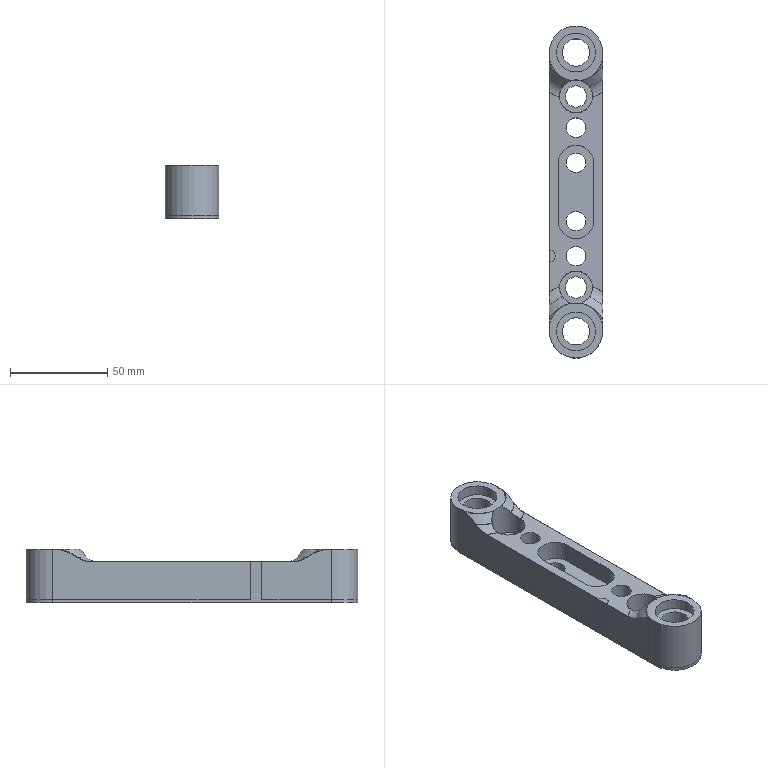NC program | NX | posted with a generic post | part box 27.4 x 170.48 x 27.5 mm
Lines 378 to 1221 of 16455:
(CURVE_DRIVE , TOOL : R3)
N688 T10 M6
N690 G54
N692 G17 G0 G90 X49.499 Y5.551 B0. C0. S4000 M3
N694 G43 Z30. H10
N696 Z-3.399
N698 G94 G1 Z-3.614 F1500.
N700 X49.462 Y5.673 Z-4.386
N702 X49.369 Y5.983 Z-5.1
N704 X49.226 Y6.459 Z-5.705
N706 X49.043 Y7.069 Z-6.161
N708 X48.832 Y7.771 Z-6.437
N710 X48.608 Y8.517 Z-6.513
N712 X48.584 Y8.595 Z-6.51
N714 X48.613 Y8.669 Z-6.507
N716 X48.657 Y8.524 Z-6.511
N718 X48.707 Y8.53 Z-6.51
N720 X48.643 Y8.744 Z-6.505
N722 X48.672 Y8.818 Z-6.502
N724 X48.756 Y8.537 Z-6.508
N726 X48.806 Y8.543 Z-6.507
N728 X48.701 Y8.893 Z-6.499
N730 X48.73 Y8.967
N732 X48.856 Y8.549 Z-6.506
N734 X48.905 Y8.555 Z-6.504
N736 X48.804 Y8.892 Z-6.496
N738 X48.759 Y9.041 Z-6.499
N740 X48.788 Y9.115 Z-6.498
N742 X48.854 Y8.892 Z-6.494
N744 X48.955 Y8.559 Z-6.498
N746 X49.004 Y8.561 Z-6.49
N748 X48.816 Y9.187 Z-6.498
N750 X48.845 Y9.256
N752 X49.053 Y8.564 Z-6.483
N754 X49.103 Y8.566 Z-6.476
N756 X49.042 Y8.769 Z-6.478
N758 X48.922 Y9.166 Z-6.495
N760 X48.875 Y9.324 Z-6.498
N762 X48.904 Y9.393
N764 X49.055 Y8.892 Z-6.482
N766 X49.114 Y8.696 Z-6.47
N768 X49.152 Y8.568 Z-6.468
N770 X49.202 Y8.571 Z-6.461
N772 X48.978 Y9.313 Z-6.494
N774 X48.934 Y9.461 Z-6.497
N776 X48.964 Y9.529
N778 X49.066 Y9.188 Z-6.489
N780 X49.251 Y8.573 Z-6.454
N782 X49.301 Y8.575 Z-6.451
N784 X49.098 Y9.252 Z-6.488
N786 X48.993 Y9.598 Z-6.497
N788 X49.023 Y9.667
N790 X49.129 Y9.315 Z-6.488
N792 X49.333 Y8.637 Z-6.451
N794 X49.351 Y8.578 Z-6.445
N796 X49.4 Y8.58 Z-6.436
N798 X49.306 Y8.892 Z-6.464
N800 X49.16 Y9.378 Z-6.487
N802 X49.053 Y9.735 Z-6.496
N804 X49.082 Y9.803
N806 X49.191 Y9.441 Z-6.486
N808 X49.356 Y8.892 Z-6.457
N810 X49.449 Y8.583 Z-6.427
N812 X49.498 Y8.586 Z-6.418
N814 X49.378 Y8.984 Z-6.46
N816 X49.155 Y9.727 Z-6.491
N818 X49.112 Y9.871 Z-6.496
N820 X49.141 Y9.939
N822 X49.253 Y9.566 Z-6.485
N824 X49.409 Y9.047 Z-6.459
N826 X49.547 Y8.588 Z-6.409
N828 X49.595 Y8.591 Z-6.4
N830 X49.504 Y8.892 Z-6.43
N832 X49.439 Y9.108 Z-6.459
N834 X49.253 Y9.727 Z-6.487
N836 X49.17 Y10.005 Z-6.496
N838 X49.198 Y10.069
N840 X49.469 Y9.168 Z-6.458
N842 X49.552 Y8.892 Z-6.421
N844 X49.642 Y8.594 Z-6.39
N846 X49.689 Y8.596 Z-6.38
N848 X49.499 Y9.228 Z-6.457
N850 X49.227 Y10.13 Z-6.496
N852 X49.256 Y10.192
N854 X49.396 Y9.727 Z-6.478
N856 X49.528 Y9.287 Z-6.456
N858 X49.647 Y8.892 Z-6.404
N860 X49.735 Y8.599 Z-6.37
N862 X49.782 Y8.598 Z-6.36
N864 X49.755 Y8.688 Z-6.375
N866 X49.693 Y8.892 Z-6.395
N868 X49.557 Y9.346 Z-6.455
N870 X49.401 Y9.865 Z-6.483
N872 X49.285 Y10.252 Z-6.496
N874 X49.313 Y10.312
N876 X49.429 Y9.923 Z-6.483
N878 X49.586 Y9.404 Z-6.454
N880 X49.739 Y8.892 Z-6.387
N882 X49.795 Y8.708 Z-6.369
N884 X49.83 Y8.59 Z-6.349
N886 X49.878 Y8.583 Z-6.338
N888 X49.834 Y8.729 Z-6.362
N890 X49.785 Y8.892 Z-6.378
N892 X49.614 Y9.462 Z-6.454
N894 X49.458 Y9.981 Z-6.483
N896 X49.341 Y10.372 Z-6.496
N898 X49.368 Y10.431
N900 X49.486 Y10.038 Z-6.483
N902 X49.642 Y9.519 Z-6.453
N904 X49.831 Y8.892 Z-6.37
N906 X49.874 Y8.749 Z-6.356
N908 X49.926 Y8.575 Z-6.327
N910 X49.973 Y8.568 Z-6.316
N912 X49.913 Y8.768 Z-6.349
N914 X49.67 Y9.576 Z-6.452
N916 X49.514 Y10.095 Z-6.483
N918 X49.396 Y10.49 Z-6.496
N920 X49.423 Y10.548
N922 X49.542 Y10.151 Z-6.483
N924 X49.698 Y9.632 Z-6.451
N926 X49.952 Y8.788 Z-6.343
N928 X50.02 Y8.561 Z-6.305
N930 X50.067 Y8.554 Z-6.294
N932 X49.99 Y8.808 Z-6.337
N934 X49.714 Y9.727 Z-6.452
N936 X49.57 Y10.207 Z-6.483
N938 X49.45 Y10.605 Z-6.496
N940 X49.477 Y10.662
N942 X49.597 Y10.263 Z-6.482
N944 X49.758 Y9.727 Z-6.448
N946 X50.029 Y8.827 Z-6.33
N948 X50.113 Y8.546 Z-6.283
N950 X50.158 Y8.539 Z-6.273
N952 X50.052 Y8.892 Z-6.329
N954 X49.78 Y9.798 Z-6.45
N956 X49.624 Y10.317 Z-6.482
N958 X49.503 Y10.719 Z-6.496
N960 X49.53 Y10.775
N962 X49.651 Y10.371 Z-6.482
N964 X49.807 Y9.852 Z-6.449
N966 X50.104 Y8.865 Z-6.318
N968 X50.204 Y8.532 Z-6.258
N970 X50.248 Y8.526 Z-6.24
N972 X50.141 Y8.884 Z-6.312
N974 X49.887 Y9.727 Z-6.429
N976 X49.834 Y9.906 Z-6.449
N978 X49.677 Y10.425 Z-6.482
N980 X49.556 Y10.83 Z-6.496
N982 X49.582 Y10.885
N984 X49.704 Y10.478 Z-6.482
N986 X49.86 Y9.959 Z-6.449
N988 X49.93 Y9.727 Z-6.423
N990 X50.181 Y8.892 Z-6.302
N992 X50.272 Y8.59 Z-6.243
N994 X50.293 Y8.519 Z-6.224
N996 X50.337 Y8.513 Z-6.208
N998 X50.304 Y8.623 Z-6.236
N1000 X50.158 Y9.109 Z-6.33
N1002 X49.972 Y9.727 Z-6.417
N1004 X49.886 Y10.013 Z-6.449
N1006 X49.73 Y10.532 Z-6.482
N1008 X49.608 Y10.939 Z-6.496
N1010 X49.635 Y10.993
N1012 X49.757 Y10.586 Z-6.482
N1014 X49.913 Y10.067 Z-6.449
N1016 X50.015 Y9.727 Z-6.411
N1018 X50.158 Y9.252 Z-6.344
N1020 X50.337 Y8.656 Z-6.23
N1022 X50.361 Y8.577 Z-6.206
N1024 X50.382 Y8.506 Z-6.192
N1026 X50.428 Y8.5 Z-6.176
N1028 X50.399 Y8.597 Z-6.194
N1030 X50.371 Y8.69 Z-6.223
N1032 X50.158 Y9.397 Z-6.358
N1034 X50.059 Y9.727 Z-6.405
N1036 X49.94 Y10.122 Z-6.449
N1038 X49.784 Y10.641 Z-6.482
N1040 X49.662 Y11.047 Z-6.496
N1042 X49.689 Y11.102
N1044 X49.852 Y10.563 Z-6.473
N1046 X49.968 Y10.177 Z-6.448
N1048 X50.103 Y9.727 Z-6.398
N1050 X50.158 Y9.543 Z-6.372
N1052 X50.404 Y8.724 Z-6.216
N1054 X50.437 Y8.616 Z-6.183
N1056 X50.474 Y8.493 Z-6.16
N1058 X50.52 Y8.486 Z-6.144
N1060 X50.475 Y8.635 Z-6.172
N1062 X50.438 Y8.758 Z-6.209
N1064 X50.147 Y9.727 Z-6.392
N1066 X49.995 Y10.232 Z-6.448
N1068 X49.839 Y10.752 Z-6.482
N1070 X49.717 Y11.158 Z-6.497
N1072 X49.744 Y11.214
N1074 X49.866 Y10.807 Z-6.482
N1076 X50.023 Y10.288 Z-6.448
N1078 X50.191 Y9.727 Z-6.382
N1080 X50.472 Y8.792 Z-6.202
N1082 X50.514 Y8.655 Z-6.16
N1084 X50.566 Y8.479 Z-6.128
N1086 X50.612 Y8.473 Z-6.111
N1088 X50.552 Y8.674 Z-6.148
N1090 X50.506 Y8.827 Z-6.195
N1092 X50.218 Y9.788 Z-6.383
N1094 X50.05 Y10.344 Z-6.448
N1096 X49.894 Y10.864 Z-6.482
N1098 X49.772 Y11.269 Z-6.497
N1100 X49.802 Y11.324 Z-6.496
N1102 X49.923 Y10.922 Z-6.482
N1104 X50.079 Y10.403 Z-6.448
N1106 X50.253 Y9.824 Z-6.379
N1108 X50.542 Y8.863 Z-6.188
N1110 X50.593 Y8.695 Z-6.136
N1112 X50.664 Y8.457 Z-6.092
N1114 X50.716 Y8.442 Z-6.073
N1116 X50.634 Y8.716 Z-6.124
N1118 X50.577 Y8.905 Z-6.182
N1120 X50.29 Y9.861 Z-6.375
N1122 X50.109 Y10.463 Z-6.447
N1124 X49.953 Y10.982 Z-6.482
N1126 X49.833 Y11.381 Z-6.496
N1128 X49.864 Y11.44
N1130 X49.983 Y11.044 Z-6.482
N1132 X50.158 Y10.463 Z-6.44
N1134 X50.328 Y9.899 Z-6.371
N1136 X50.379 Y9.727 Z-6.331
N1138 X50.608 Y8.967 Z-6.181
N1140 X50.677 Y8.737 Z-6.111
N1142 X50.77 Y8.426 Z-6.051
N1144 X50.824 Y8.411 Z-6.021
N1146 X50.794 Y8.51 Z-6.052
N1148 X50.72 Y8.759 Z-6.098
N1150 X50.638 Y9.029 Z-6.18
N1152 X50.428 Y9.727 Z-6.318
N1154 X50.365 Y9.937 Z-6.366
N1156 X50.17 Y10.587 Z-6.447
N1158 X50.014 Y11.106 Z-6.482
N1160 X49.896 Y11.498 Z-6.496
N1162 X49.927 Y11.556
N1164 X50.044 Y11.167 Z-6.483
N1166 X50.2 Y10.647 Z-6.447
N1168 X50.402 Y9.974 Z-6.362
N1170 X50.477 Y9.727 Z-6.305
N1172 X50.668 Y9.089 Z-6.179
N1174 X50.761 Y8.78 Z-6.086
N1176 X50.824 Y8.57 Z-6.047
N1178 X50.877 Y8.395 Z-5.991
N1180 X50.93 Y8.38 Z-5.961
N1182 X50.854 Y8.631 Z-6.042
N1184 X50.803 Y8.801 Z-6.073
N1186 X50.698 Y9.15 Z-6.178
N1188 X50.525 Y9.727 Z-6.292
N1190 X50.439 Y10.012 Z-6.358
N1192 X50.23 Y10.708 Z-6.448
N1194 X50.074 Y11.227 Z-6.483
N1196 X49.958 Y11.613 Z-6.496
N1198 X49.989 Y11.67
N1200 X50.104 Y11.288 Z-6.483
N1202 X50.26 Y10.768 Z-6.448
N1204 X50.322 Y10.563 Z-6.417
N1206 X50.476 Y10.049 Z-6.353
N1208 X50.573 Y9.727 Z-6.279
N1210 X50.728 Y9.21 Z-6.177
N1212 X50.845 Y8.822 Z-6.061
N1214 X50.884 Y8.691 Z-6.037
N1216 X50.982 Y8.364 Z-5.932
N1218 X51.039 Y8.337 Z-5.901
N1220 X50.914 Y8.752 Z-6.031
N1222 X50.887 Y8.843 Z-6.048
N1224 X50.758 Y9.271 Z-6.176
N1226 X50.621 Y9.727 Z-6.266
N1228 X50.513 Y10.086 Z-6.349
N1230 X50.37 Y10.563 Z-6.408
N1232 X50.29 Y10.829 Z-6.448
N1234 X50.134 Y11.348 Z-6.483
N1236 X50.02 Y11.727 Z-6.496
N1238 X50.051 Y11.782
N1240 X50.163 Y11.408 Z-6.483
N1242 X50.319 Y10.889 Z-6.448
N1244 X50.418 Y10.563 Z-6.399
N1246 X50.55 Y10.123 Z-6.345
N1248 X50.669 Y9.727 Z-6.254
N1250 X50.788 Y9.331 Z-6.175
N1252 X50.928 Y8.864 Z-6.036
N1254 X50.944 Y8.812 Z-6.026
N1256 X51.096 Y8.307 Z-5.869
N1258 X51.147 Y8.279 Z-5.833
N1260 X51.127 Y8.347 Z-5.861
N1262 X50.966 Y8.883 Z-6.025
N1264 X50.815 Y9.385 Z-6.174
N1266 X50.712 Y9.727 Z-6.242
N1268 X50.583 Y10.157 Z-6.341
N1270 X50.461 Y10.563 Z-6.391
N1272 X50.346 Y10.943 Z-6.449
N1274 X50.19 Y11.463 Z-6.483
N1276 X50.079 Y11.832 Z-6.496
N1278 X50.11 Y11.886
N1280 X50.22 Y11.522 Z-6.483
N1282 X50.376 Y11.003 Z-6.449
N1284 X50.508 Y10.563 Z-6.382
N1286 X50.619 Y10.194 Z-6.337
N1288 X50.759 Y9.727 Z-6.23
N1290 X50.844 Y9.445 Z-6.174
N1292 X51.156 Y8.406 Z-5.857
N1294 X51.203 Y8.249 Z-5.791
N1296 X51.26 Y8.219 Z-5.75
N1298 X51.185 Y8.465 Z-5.853
N1300 X51.057 Y8.892 Z-5.985
N1302 X51.029 Y8.985 Z-6.018
N1304 X50.873 Y9.504 Z-6.173
N1306 X50.806 Y9.727 Z-6.217
N1308 X50.655 Y10.23 Z-6.333
N1310 X50.555 Y10.563 Z-6.374
N1312 X50.405 Y11.062 Z-6.449
N1314 X50.249 Y11.581 Z-6.483
N1316 X50.141 Y11.94 Z-6.496
N1318 X50.17 Y11.992
N1320 X50.278 Y11.64 Z-6.483
N1322 X50.434 Y11.121 Z-6.449
N1324 X50.602 Y10.563 Z-6.365
N1326 X50.691 Y10.267 Z-6.328
N1328 X50.853 Y9.727 Z-6.204
N1330 X50.903 Y9.563 Z-6.172
N1332 X51.059 Y9.044 Z-6.018
N1334 X51.104 Y8.892 Z-5.963
N1336 X51.215 Y8.525 Z-5.849
N1338 X51.316 Y8.188 Z-5.709
N1340 X51.372 Y8.158 Z-5.668
N1342 X51.244 Y8.584 Z-5.845
N1344 X51.151 Y8.892 Z-5.94
N1346 X51.088 Y9.103 Z-6.017
N1348 X50.932 Y9.622 Z-6.171
N1350 X50.727 Y10.303 Z-6.324
N1352 X50.649 Y10.563 Z-6.356
N1354 X50.464 Y11.18 Z-6.45
N1356 X50.307 Y11.7 Z-6.483
N1358 X50.202 Y12.049 Z-6.496
N1360 X50.233 Y12.103
N1362 X50.337 Y11.759 Z-6.484
N1364 X50.493 Y11.24 Z-6.45
N1366 X50.696 Y10.563 Z-6.347
N1368 X50.763 Y10.34 Z-6.32
N1370 X50.961 Y9.682 Z-6.17
N1372 X51.117 Y9.162 Z-6.016
N1374 X51.198 Y8.892 Z-5.918
N1376 X51.273 Y8.643 Z-5.841
N1378 X51.428 Y8.128 Z-5.628
N1380 X51.486 Y8.09 Z-5.576
N1382 X51.459 Y8.183 Z-5.623
N1384 X51.303 Y8.702 Z-5.837
N1386 X51.245 Y8.892 Z-5.896
N1388 X51.146 Y9.222 Z-6.016
N1390 X50.99 Y9.741 Z-6.169
N1392 X50.799 Y10.376 Z-6.316
N1394 X50.743 Y10.563 Z-6.339
N1396 X50.522 Y11.299 Z-6.45
N1398 X50.366 Y11.818 Z-6.484
N1400 X50.264 Y12.157 Z-6.496
N1402 X50.294 Y12.21
N1404 X50.394 Y11.876 Z-6.484
N1406 X50.55 Y11.356 Z-6.45
N1408 X50.834 Y10.412 Z-6.312
N1410 X51.019 Y9.798 Z-6.169
N1412 X51.175 Y9.279 Z-6.015
N1414 X51.291 Y8.892 Z-5.874
N1416 X51.331 Y8.76 Z-5.834
N1418 X51.487 Y8.24 Z-5.62
N1420 X51.546 Y8.045 Z-5.52
N1422 X51.606 Y7.996 Z-5.461
N1424 X51.516 Y8.298 Z-5.617
N1426 X51.36 Y8.818 Z-5.83
N1428 X51.203 Y9.337 Z-6.014
N1430 X51.047 Y9.856 Z-6.169
N1432 X50.87 Y10.447 Z-6.308
N1434 X50.579 Y11.414 Z-6.451
N1436 X50.423 Y11.934 Z-6.484
N1438 X50.324 Y12.263 Z-6.496
N1440 X50.354 Y12.316
N1442 X50.452 Y11.992 Z-6.484
N1444 X50.63 Y11.398 Z-6.442
N1446 X50.905 Y10.483 Z-6.303
N1448 X51.076 Y9.914 Z-6.17
N1450 X51.232 Y9.395 Z-6.014
N1452 X51.388 Y8.876 Z-5.826
N1454 X51.544 Y8.357 Z-5.614
N1456 X51.667 Y7.948 Z-5.402
N1458 X51.728 Y7.899 Z-5.344
N1460 X51.573 Y8.415 Z-5.611
N1462 X51.417 Y8.934 Z-5.824
N1464 X51.261 Y9.453 Z-6.013
N1466 X51.105 Y9.973 Z-6.17
N1468 X50.941 Y10.519 Z-6.299
N1470 X50.676 Y11.398 Z-6.436
N1472 X50.637 Y11.53 Z-6.452
N1474 X50.48 Y12.05 Z-6.484
N1476 X50.384 Y12.37 Z-6.496
N1478 X50.414 Y12.422
N1480 X50.571 Y11.901 Z-6.471
N1482 X50.665 Y11.588 Z-6.452
N1484 X50.722 Y11.398 Z-6.43
N1486 X50.976 Y10.555 Z-6.295
N1488 X51.133 Y10.03 Z-6.17
N1490 X51.289 Y9.511 Z-6.012
N1492 X51.445 Y8.992 Z-5.823
N1494 X51.602 Y8.472 Z-5.609
N1496 X51.788 Y7.851 Z-5.285
N1498 X51.848 Y7.802 Z-5.222
N1500 X51.771 Y8.059 Z-5.366
N1502 X51.63 Y8.529 Z-5.606
N1504 X51.473 Y9.048 Z-5.823
N1506 X51.317 Y9.567 Z-6.012
N1508 X51.161 Y10.087 Z-6.17
N1510 X50.984 Y10.678 Z-6.308
N1512 X50.767 Y11.398 Z-6.424
N1514 X50.693 Y11.645 Z-6.453
N1516 X50.537 Y12.164 Z-6.485
N1518 X50.444 Y12.474 Z-6.496
N1520 X50.473 Y12.525
N1522 X50.562 Y12.227 Z-6.485
N1524 X50.72 Y11.7 Z-6.453
N1526 X50.811 Y11.398 Z-6.417
N1528 X50.984 Y10.825 Z-6.326
N1530 X51.062 Y10.563 Z-6.271
N1532 X51.189 Y10.142 Z-6.17
N1534 X51.345 Y9.623 Z-6.011
N1536 X51.501 Y9.104 Z-5.822
N1538 X51.564 Y8.892 Z-5.728
N1540 X51.657 Y8.584 Z-5.603
N1542 X51.813 Y8.065 Z-5.338
N1544 X51.907 Y7.754 Z-5.157
N1546 X51.965 Y7.705 Z-5.086
N1548 X51.84 Y8.12 Z-5.336
N1550 X51.684 Y8.64 Z-5.6
N1552 X51.608 Y8.892 Z-5.703
N1554 X51.528 Y9.159 Z-5.821
N1556 X51.357 Y9.727 Z-6.025
N1558 X51.216 Y10.197 Z-6.17
N1560 X51.078 Y10.658 Z-6.282
N1562 X50.984 Y10.97 Z-6.343
N1564 X50.855 Y11.398 Z-6.411
N1566 X50.748 Y11.755 Z-6.454
N1568 X50.592 Y12.275 Z-6.485
N1570 X50.502 Y12.574 Z-6.497
N1572 X50.531 Y12.623
N1574 X50.648 Y12.233 Z-6.48
N1576 X50.775 Y11.81 Z-6.454
N1578 X50.899 Y11.398 Z-6.406
N1580 X50.984 Y11.116 Z-6.36
N1582 X51.111 Y10.692 Z-6.277
N1584 X51.243 Y10.252 Z-6.17
N1586 X51.399 Y9.733 Z-6.01
N1588 X51.555 Y9.214 Z-5.82
N1590 X51.652 Y8.892 Z-5.678
N1592 X51.711 Y8.695 Z-5.598
N1594 X51.868 Y8.175 Z-5.333
N1596 X51.977 Y7.81 Z-5.115
N1598 X52.024 Y7.655 Z-5.014
N1600 X52.082 Y7.605 Z-4.942
N1602 X52.011 Y7.844 Z-5.098
N1604 X51.895 Y8.23 Z-5.33
N1606 X51.739 Y8.749 Z-5.595
N1608 X51.582 Y9.269 Z-5.819
N1610 X51.426 Y9.788 Z-6.01
N1612 X51.27 Y10.307 Z-6.17
N1614 X51.145 Y10.725 Z-6.272
N1616 X50.984 Y11.261 Z-6.378
N1618 X50.943 Y11.398 Z-6.4
N1620 X50.802 Y11.865 Z-6.455
N1622 X50.646 Y12.385 Z-6.486
N1624 X50.56 Y12.672 Z-6.497
N1626 X50.589 Y12.72
N1628 X50.735 Y12.233 Z-6.474
N1630 X50.829 Y11.92 Z-6.455
N1632 X50.986 Y11.4 Z-6.394
N1634 X51.178 Y10.759 Z-6.268
N1636 X51.297 Y10.362 Z-6.17
N1638 X51.453 Y9.843 Z-6.01
N1640 X51.61 Y9.324 Z-5.819
N1642 X51.766 Y8.804 Z-5.592
N1644 X51.922 Y8.285 Z-5.328
N1646 X52.044 Y7.877 Z-5.081
N1648 X52.141 Y7.556 Z-4.87
N1650 X52.2 Y7.505 Z-4.797
N1652 X52.078 Y7.911 Z-5.064
N1654 X51.949 Y8.34 Z-5.325
N1656 X51.783 Y8.892 Z-5.603
N1658 X51.637 Y9.378 Z-5.818
N1660 X51.481 Y9.898 Z-6.011
N1662 X51.325 Y10.417 Z-6.17
N1664 X51.212 Y10.793 Z-6.263
N1666 X51.019 Y11.433 Z-6.391
N1668 X50.856 Y11.975 Z-6.456
N1670 X50.618 Y12.768 Z-6.497
N1672 X50.648 Y12.815 Z-6.496
N1674 X50.884 Y12.03 Z-6.456
N1676 X51.053 Y11.468 Z-6.388
N1678 X51.245 Y10.827 Z-6.259
N1680 X51.352 Y10.472 Z-6.17
N1682 X51.508 Y9.953 Z-6.011
N1684 X51.664 Y9.434 Z-5.817
N1686 X51.827 Y8.892 Z-5.575
N1688 X51.976 Y8.395 Z-5.322
N1690 X52.111 Y7.945 Z-5.047
N1692 X52.26 Y7.452 Z-4.723
N1694 X52.318 Y7.4 Z-4.65
N1696 X52.144 Y7.978 Z-5.03
N1698 X52.002 Y8.448 Z-5.32
N1700 X51.846 Y8.967 Z-5.587
N1702 X51.69 Y9.487 Z-5.816
N1704 X51.534 Y10.006 Z-6.012
N1706 X51.367 Y10.563 Z-6.179
N1708 X51.277 Y10.86 Z-6.254
N1710 X51.116 Y11.398 Z-6.36
N1712 X51.085 Y11.5 Z-6.385
N1714 X50.91 Y12.083 Z-6.457
N1716 X50.676 Y12.86 Z-6.496
N1718 X50.706 Y12.907
N1720 X50.937 Y12.139 Z-6.457
N1722 X51.119 Y11.534 Z-6.382
N1724 X51.16 Y11.398 Z-6.349
N1726 X51.311 Y10.894 Z-6.25
N1728 X51.405 Y10.581 Z-6.17
N1730 X51.561 Y10.061 Z-6.012
N1732 X51.718 Y9.542 Z-5.816
N1734 X51.874 Y9.023 Z-5.586
N1736 X52.03 Y8.503 Z-5.317
N1738 X52.177 Y8.012 Z-5.013
N1740 X52.38 Y7.339 Z-4.572
N1742 X52.441 Y7.28 Z-4.497
N1744 X52.207 Y8.057 Z-5.002
N1746 X52.057 Y8.558 Z-5.315
N1748 X51.901 Y9.078 Z-5.585
N1750 X51.745 Y9.597 Z-5.815
N1752 X51.589 Y10.116 Z-6.012
N1754 X51.432 Y10.635 Z-6.171
N1756 X51.345 Y10.928 Z-6.245
N1758 X51.203 Y11.398 Z-6.338
N1760 X51.152 Y11.568 Z-6.379
N1762 X50.964 Y12.193 Z-6.458
N1764 X50.736 Y12.954 Z-6.496
N1766 X50.765 Y12.999
N1768 X50.995 Y12.233 Z-6.456
N1770 X51.185 Y11.601 Z-6.376
N1772 X51.246 Y11.398 Z-6.327
N1774 X51.377 Y10.961 Z-6.241
N1776 X51.459 Y10.689 Z-6.172
N1778 X51.615 Y10.17 Z-6.013
N1780 X51.771 Y9.65 Z-5.814
N1782 X51.927 Y9.131 Z-5.584
N1784 X52.083 Y8.612 Z-5.312
N1786 X52.25 Y8.057 Z-4.964
N1788 X52.477 Y7.302 Z-4.469
N1790 X52.501 Y7.222 Z-4.424
N1792 X52.56 Y7.165 Z-4.349
N1794 X52.527 Y7.277 Z-4.414
N1796 X52.266 Y8.145 Z-4.987
N1798 X52.109 Y8.665 Z-5.31
N1800 X51.953 Y9.184 Z-5.583
N1802 X51.79 Y9.727 Z-5.822
N1804 X51.641 Y10.223 Z-6.013
N1806 X51.485 Y10.742 Z-6.173
N1808 X51.41 Y10.993 Z-6.236
N1810 X51.288 Y11.398 Z-6.316
N1812 X51.217 Y11.634 Z-6.373
N1814 X51.025 Y12.274 Z-6.456
N1816 X50.793 Y13.044 Z-6.496
N1818 X50.822 Y13.089
N1820 X51.057 Y12.307 Z-6.455
N1822 X51.249 Y11.666 Z-6.371
N1824 X51.33 Y11.398 Z-6.305
N1826 X51.442 Y11.026 Z-6.232
N1828 X51.511 Y10.795 Z-6.173
N1830 X51.667 Y10.276 Z-6.013
N1832 X51.832 Y9.727 Z-5.8
N1834 X51.979 Y9.237 Z-5.582
N1836 X52.136 Y8.718 Z-5.307
N1838 X52.292 Y8.198 Z-4.985
N1840 X52.334 Y8.057 Z-4.887
N1842 X52.585 Y7.222 Z-4.343
N1844 X52.62 Y7.107 Z-4.273
N1846 X52.68 Y7.048 Z-4.197
N1848 X52.626 Y7.227 Z-4.305
N1850 X52.376 Y8.057 Z-4.848
N1852 X52.318 Y8.252 Z-4.984
N1854 X52.162 Y8.771 Z-5.305
N1856 X52.006 Y9.29 Z-5.581
N1858 X51.85 Y9.81 Z-5.814
N1860 X51.694 Y10.329 Z-6.014
N1862 X51.538 Y10.848 Z-6.174
N1864 X51.474 Y11.059 Z-6.228
N1866 X51.372 Y11.398 Z-6.294
N1868 X51.282 Y11.699 Z-6.368
N1870 X51.089 Y12.34 Z-6.453
N1872 X50.85 Y13.134 Z-6.496
N1874 X50.879 Y13.18
N1876 X51.122 Y12.373 Z-6.451
N1878 X51.164 Y12.233 Z-6.428
N1880 X51.314 Y11.732 Z-6.365
N1882 X51.415 Y11.398 Z-6.283
N1884 X51.507 Y11.092 Z-6.223
N1886 X51.564 Y10.902 Z-6.175
N1888 X51.72 Y10.382 Z-6.014
N1890 X51.876 Y9.863 Z-5.815
N1892 X52.032 Y9.344 Z-5.58
N1894 X52.188 Y8.824 Z-5.302
N1896 X52.344 Y8.305 Z-4.982
N1898 X52.419 Y8.057 Z-4.808
N1900 X52.685 Y7.171 Z-4.231
N1902 X52.74 Y6.99 Z-4.12
N1904 X52.8 Y6.931 Z-4.044
N1906 X52.712 Y7.222 Z-4.223
N1908 X52.461 Y8.057 Z-4.769
N1910 X52.371 Y8.358 Z-4.98
N1912 X52.21 Y8.892 Z-5.307
N1914 X52.059 Y9.397 Z-5.579
N1916 X51.903 Y9.916 Z-5.816
N1918 X51.746 Y10.436 Z-6.015
N1920 X51.59 Y10.955 Z-6.176
N1922 X51.539 Y11.125 Z-6.219
N1924 X51.457 Y11.398 Z-6.272
N1926 X51.347 Y11.765 Z-6.362
N1928 X51.206 Y12.233 Z-6.421
N1930 X51.154 Y12.405 Z-6.45
N1932 X50.908 Y13.225 Z-6.496
N1934 X50.937 Y13.271
N1936 X51.187 Y12.438 Z-6.448
N1938 X51.249 Y12.233 Z-6.414
N1940 X51.379 Y11.798 Z-6.359
N1942 X51.5 Y11.398 Z-6.262
N1944 X51.572 Y11.158 Z-6.214
N1946 X51.617 Y11.008 Z-6.176
N1948 X51.773 Y10.489 Z-6.015
N1950 X51.929 Y9.97 Z-5.817
N1952 X52.002 Y9.727 Z-5.701
N1954 X52.085 Y9.45 Z-5.578
N1956 X52.253 Y8.892 Z-5.274
N1958 X52.397 Y8.412 Z-4.978
N1960 X52.504 Y8.057 Z-4.73
N1962 X52.807 Y7.048 Z-4.074
N1964 X52.86 Y6.873 Z-3.967
N1966 X52.918 Y6.816 Z-3.893
N1968 X52.796 Y7.222 Z-4.145
N1970 X52.545 Y8.057 Z-4.692
N1972 X52.423 Y8.464 Z-4.977
N1974 X52.267 Y8.983 Z-5.298
N1976 X52.111 Y9.502 Z-5.577
N1978 X52.043 Y9.727 Z-5.677
N1980 X51.955 Y10.022 Z-5.818
N1982 X51.798 Y10.541 Z-6.015
N1984 X51.642 Y11.06 Z-6.177
N1986 X51.603 Y11.19 Z-6.21
N1988 X51.541 Y11.398 Z-6.251
N1990 X51.411 Y11.83 Z-6.357
N1992 X51.29 Y12.233 Z-6.407
N1994 X51.219 Y12.47 Z-6.447
N1996 X51.018 Y13.137 Z-6.49
N1998 X50.965 Y13.315 Z-6.496
N2000 X50.994 Y13.36
N2002 X51.081 Y13.068 Z-6.481
N2004 X51.251 Y12.503 Z-6.445
N2006 X51.332 Y12.233 Z-6.4
N2008 X51.444 Y11.863 Z-6.354
N2010 X51.583 Y11.398 Z-6.24
N2012 X51.636 Y11.223 Z-6.206
N2014 X51.669 Y11.114 Z-6.178
N2016 X51.825 Y10.594 Z-6.016
N2018 X51.981 Y10.075 Z-5.819
N2020 X52.137 Y9.556 Z-5.577
N2022 X52.293 Y9.036 Z-5.297
N2024 X52.449 Y8.517 Z-4.975
N2026 X52.587 Y8.057 Z-4.653
N2028 X52.838 Y7.222 Z-4.106
N2030 X52.978 Y6.757 Z-3.816
N2032 X53.036 Y6.701 Z-3.743
N2034 X52.879 Y7.222 Z-4.068
N2036 X52.628 Y8.057 Z-4.615
N2038 X52.474 Y8.568 Z-4.973
N2040 X52.318 Y9.087 Z-5.296
N2042 X52.162 Y9.607 Z-5.576
N2044 X52.006 Y10.126 Z-5.82
N2046 X51.85 Y10.645 Z-6.018
N2048 X51.694 Y11.165 Z-6.179
N2050 X51.624 Y11.398 Z-6.23
N2052 X51.475 Y11.894 Z-6.351
N2054 X51.373 Y12.233 Z-6.394
N2056 X51.282 Y12.535 Z-6.444
N2058 X51.07 Y13.242 Z-6.491
N2060 X51.021 Y13.403 Z-6.497
N2062 X51.05 Y13.449
N2064 X51.096 Y13.295 Z-6.492
N2066 X51.315 Y12.568 Z-6.442
N2068 X51.415 Y12.233 Z-6.387
N2070 X51.507 Y11.927 Z-6.348
N2072 X51.666 Y11.398 Z-6.219
N2074 X51.72 Y11.218 Z-6.18
N2076 X51.876 Y10.699 Z-6.019
N2078 X52.033 Y10.179 Z-5.82
N2080 X52.189 Y9.66 Z-5.575
N2082 X52.345 Y9.141 Z-5.296
N2084 X52.501 Y8.621 Z-4.971
N2086 X52.686 Y8.005 Z-4.542
N2088 X52.921 Y7.222 Z-4.028
N2090 X53.099 Y6.632 Z-3.66
N2092 X53.162 Y6.559 Z-3.576
N2094 X52.963 Y7.222 Z-3.99
N2096 X52.712 Y8.057 Z-4.539
N2098 X52.527 Y8.674 Z-4.97
N2100 X52.37 Y9.193 Z-5.295
N2102 X52.21 Y9.727 Z-5.581
N2104 X52.058 Y10.231 Z-5.821
N2106 X51.902 Y10.751 Z-6.02
N2108 X51.731 Y11.319 Z-6.193
N2110 X51.539 Y11.959 Z-6.345
N2112 X51.457 Y12.233 Z-6.38
N2114 X51.346 Y12.6 Z-6.441
N2116 X51.122 Y13.347 Z-6.493
N2118 X51.078 Y13.493 Z-6.498
N2120 X51.107 Y13.538 Z-6.499
N2122 X51.148 Y13.401 Z-6.494
N2124 X51.379 Y12.633 Z-6.439
N2126 X51.499 Y12.233 Z-6.373
N2128 X51.571 Y11.992 Z-6.342
N2130 X51.772 Y11.323 Z-6.181
N2132 X51.929 Y10.804 Z-6.022
N2134 X52.085 Y10.285 Z-5.822
N2136 X52.252 Y9.727 Z-5.553
N2138 X52.397 Y9.246 Z-5.294
N2140 X52.553 Y8.727 Z-4.968
N2142 X52.806 Y7.884 Z-4.384
N2144 X53.005 Y7.222 Z-3.95
N2146 X53.232 Y6.469 Z-3.48
N2148 X53.301 Y6.379 Z-3.385
N2150 X53.047 Y7.222 Z-3.911
N2152 X52.796 Y8.057 Z-4.462
N2154 X52.579 Y8.78 Z-4.966
N2156 X52.423 Y9.299 Z-5.294
N2158 X52.267 Y9.819 Z-5.576
N2160 X52.111 Y10.338 Z-5.823
N2162 X51.955 Y10.857 Z-6.023
N2164 X51.792 Y11.398 Z-6.187
N2166 X51.604 Y12.025 Z-6.34
N2168 X51.541 Y12.233 Z-6.366
N2170 X51.411 Y12.665 Z-6.438
N2172 X51.29 Y13.068 Z-6.463
N2174 X51.174 Y13.454 Z-6.495
N2176 X51.135 Y13.583 Z-6.499
N2178 X51.164 Y13.628 Z-6.5
N2180 X51.2 Y13.506 Z-6.495
N2182 X51.332 Y13.068 Z-6.459
N2184 X51.443 Y12.698 Z-6.436
N2186 X51.583 Y12.233 Z-6.359
N2188 X51.636 Y12.058 Z-6.337
N2190 X51.834 Y11.398 Z-6.173
N2192 X51.981 Y10.91 Z-6.024
N2194 X52.137 Y10.391 Z-5.824
N2196 X52.293 Y9.871 Z-5.578
N2198 X52.336 Y9.727 Z-5.495
N2200 X52.449 Y9.352 Z-5.293
N2202 X52.605 Y8.833 Z-4.964
N2204 X52.838 Y8.057 Z-4.424
N2206 X53.089 Y7.222 Z-3.872
N2208 X53.288 Y6.561 Z-3.455
N2210 X53.369 Y6.29 Z-3.291
N2212 X53.438 Y6.201 Z-3.197
N2214 X53.348 Y6.501 Z-3.378
N2216 X53.131 Y7.222 Z-3.833
N2218 X52.88 Y8.057 Z-4.386
N2220 X52.631 Y8.885 Z-4.963
N2222 X52.475 Y9.405 Z-5.292
N2224 X52.378 Y9.727 Z-5.466
N2226 X52.319 Y9.924 Z-5.579
N2228 X52.163 Y10.443 Z-5.825
N2230 X52.007 Y10.963 Z-6.026
N2232 X51.851 Y11.482 Z-6.185
N2234 X51.668 Y12.09 Z-6.334
N2236 X51.625 Y12.233 Z-6.352
N2238 X51.476 Y12.73 Z-6.435
N2240 X51.374 Y13.068 Z-6.456
N2242 X51.226 Y13.559 Z-6.496
N2244 X51.192 Y13.673 Z-6.5
N2246 X51.211 Y13.699
N2248 X51.225 Y13.702
N2250 X51.508 Y12.763 Z-6.433
N2252 X51.7 Y12.122 Z-6.331
N2254 X51.877 Y11.534 Z-6.187
N2256 X52.033 Y11.015 Z-6.027
N2258 X52.189 Y10.496 Z-5.826
N2260 X52.345 Y9.976 Z-5.581
N2262 X52.42 Y9.727 Z-5.437
N2264 X52.501 Y9.457 Z-5.292
N2266 X52.671 Y8.892 Z-4.93
N2268 X52.922 Y8.057 Z-4.348
N2270 X53.173 Y7.222 Z-3.794
N2272 X53.408 Y6.44 Z-3.3
N2274 X53.506 Y6.113 Z-3.103
N2276 X53.575 Y6.024 Z-3.01
N2278 X53.466 Y6.387 Z-3.228
N2280 X53.215 Y7.222 Z-3.755
N2282 X52.964 Y8.057 Z-4.31
N2284 X52.683 Y8.99 Z-4.961
N2286 X52.527 Y9.51 Z-5.291
N2288 X52.462 Y9.727 Z-5.408
N2290 X52.371 Y10.029 Z-5.583
N2292 X52.215 Y10.548 Z-5.827
N2294 X52.059 Y11.068 Z-6.028
N2296 X51.903 Y11.587 Z-6.189
N2298 X51.732 Y12.155 Z-6.328
N2300 X51.54 Y12.795 Z-6.432
N2302 X51.264 Y13.712 Z-6.499
N2304 X51.303 Y13.721
N2306 X51.572 Y12.828 Z-6.43
N2308 X51.764 Y12.187 Z-6.326
N2310 X51.929 Y11.64 Z-6.191
N2312 X52.085 Y11.12 Z-6.03
N2314 X52.253 Y10.563 Z-5.81
N2316 X52.397 Y10.082 Z-5.584
N2318 X52.504 Y9.727 Z-5.379
N2320 X52.553 Y9.563 Z-5.29
N2322 X52.709 Y9.043 Z-4.96
N2324 X53.006 Y8.057 Z-4.272
N2326 X53.257 Y7.222 Z-3.716
N2328 X53.508 Y6.387 Z-3.189
N2330 X53.643 Y5.935 Z-2.916
N2332 X53.701 Y5.861 Z-2.838
N2334 X53.543 Y6.387 Z-3.156
N2336 X53.292 Y7.222 Z-3.683
N2338 X53.041 Y8.057 Z-4.24
N2340 X52.731 Y9.088 Z-4.96
N2342 X52.575 Y9.607 Z-5.29
N2344 X52.419 Y10.126 Z-5.585
N2346 X52.263 Y10.645 Z-5.83
N2348 X52.107 Y11.165 Z-6.031
N2350 X51.951 Y11.684 Z-6.193
N2352 X51.786 Y12.233 Z-6.326
N2354 X51.599 Y12.855 Z-6.429
N2356 X51.336 Y13.729 Z-6.496
N2358 X51.363 Y13.736 Z-6.495
N2360 X51.621 Y12.878 Z-6.428
N2362 X51.813 Y12.24 Z-6.322
N2364 X51.969 Y11.72 Z-6.194
N2366 X52.125 Y11.201 Z-6.032
N2368 X52.281 Y10.682 Z-5.832